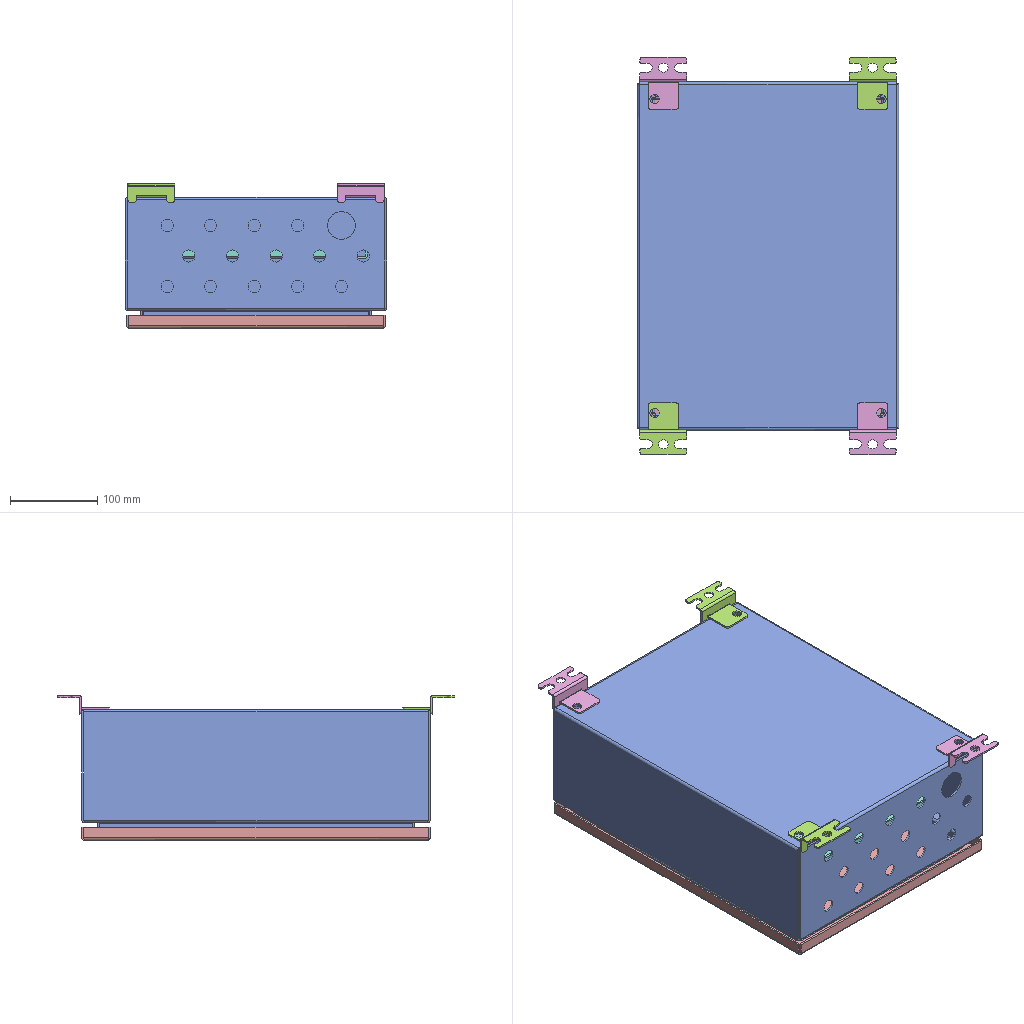Assembly | SolidWorks | 5 different items | 7 placed | box 300 x 456 x 166 mm
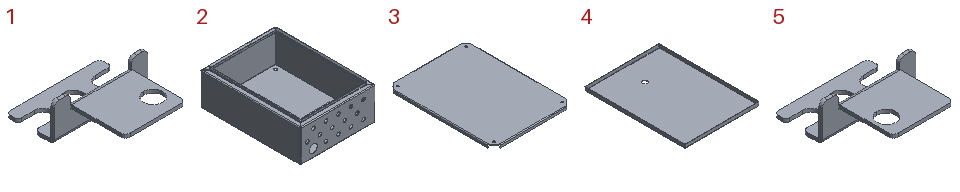Parts list (item | quantity | size | volume | features):
1 | x2 | 54 x 59.5 x 21 mm | 5826 mm3 | features Fillet 3, EdgeFlange 2, ICE 2, Cut 1, FlatPattern 1, SMBaseFlange 1, SheetMetal 1
2 | x1 | 300 x 400 x 144.964 mm | 665331 mm3 | features EdgeFlange 7, 3DProfileFeature 1, Cut 1, FlatPattern 1, HoleWzd 1, ICE 1, SMBaseFlange 1, SheetMetal 1, SketchPattern 1
3 | x1 | 255 x 345 x 10 mm | 189359 mm3 | features Chamfer 1, EdgeFlange 1, FlatPattern 1, ICE 1, SMBaseFlange 1, SheetMetal 1
4 | x1 | 297 x 400 x 15 mm | 270369 mm3 | features EdgeFlange 1, FlatPattern 1, ICE 1, SMBaseFlange 1, SheetMetal 1
5 | x2 | 54 x 59.5 x 21 mm | 5826 mm3 | features Fillet 3, EdgeFlange 2, ICE 2, Cut 1, FlatPattern 1, SMBaseFlange 1, SheetMetal 1
Mates (type | each side: item.copy, entity, surface, feature):
Coincident | 2.1 plane | assembly plane | 3 times
Coincident | 4.1 plane | assembly plane | 2 times
DistanceDim | 2.1 face plane Edge-Flange2 | 4.1 face plane Edge-Flange1
Coincident | 2.1 face plane Edge-Flange1 | 5.1 face plane Edge-Flange1
Coincident | 2.1 face plane Base-Flange1 | 5.1 face plane Edge-Flange3
DistanceDim | 5.1 face plane Edge-Flange1 | 2.1 face plane Edge-Flange1
Coincident | 2.1 face plane Edge-Flange1 | 1.1 face plane Edge-Flange1
Coincident | 5.1 face plane Base-Flange1 | 1.1 face plane Base-Flange1
DistanceDim | 1.1 face plane Edge-Flange1 | 2.1 face plane Edge-Flange1
Coincident | 2.1 face plane Edge-Flange1 | 1.2 face plane Edge-Flange1
Coincident | 2.1 face plane Base-Flange1 | 1.2 face plane Edge-Flange3
DistanceDim | 1.2 face plane Base-Flange1 | 2.1 face plane Edge-Flange1
Coincident | 2.1 face plane Edge-Flange1 | 5.2 face plane Edge-Flange1
Coincident | 2.1 face plane Base-Flange1 | 5.2 face plane Edge-Flange3
DistanceDim | 2.1 face plane Edge-Flange1 | 5.2 face plane Edge-Flange1
Parallel | 3.1 face plane Base-Flange1 | assembly plane
Coincident | 3.1 plane | assembly plane | 2 times